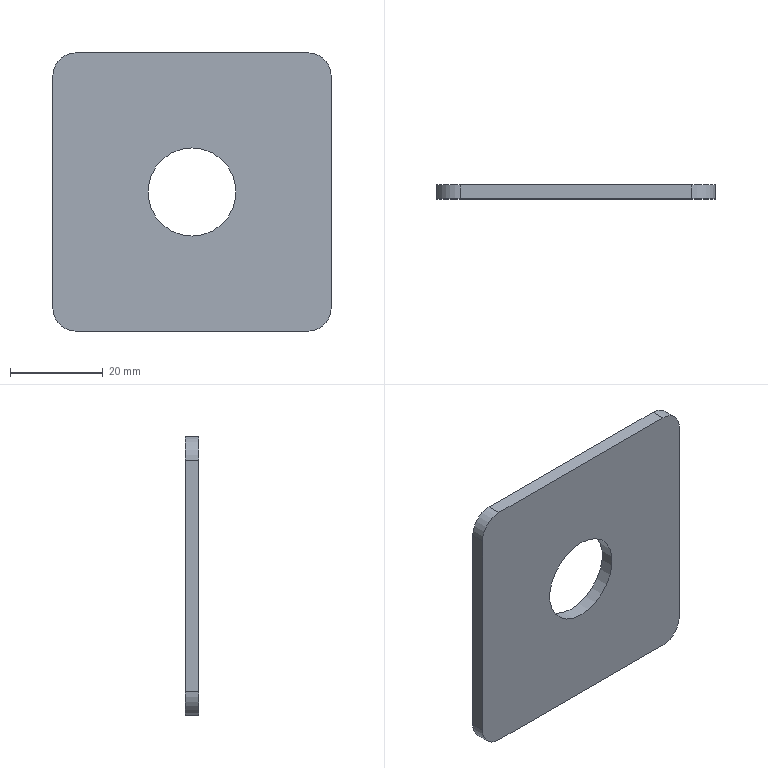Part | STEP file | JBJ-P-1006-04 | 1 solid | 11 faces | box 60 x 3 x 60 mm | volume 9885 mm3 | plane 6 | cylinder 5 | commonest cylinder face diameters 10 x4 19 x1
STEP:
#1=CARTESIAN_POINT('',(60.,3.,55.));
#2=VERTEX_POINT('',#1);
#3=CARTESIAN_POINT('',(60.,3.,5.));
#4=VERTEX_POINT('',#3);
#5=CARTESIAN_POINT('',(60.,3.,0.));
#6=DIRECTION('',(0.,0.,-1.));
#7=VECTOR('',#6,1000.);
#8=LINE('',#5,#7);
#9=EDGE_CURVE('',#2,#4,#8,.T.);
#10=ORIENTED_EDGE('',*,*,#9,.T.);
#11=CARTESIAN_POINT('',(55.,3.,0.));
#12=VERTEX_POINT('',#11);
#13=CARTESIAN_POINT('',(55.,3.,5.));
#14=DIRECTION('',(0.,1.,0.));
#15=DIRECTION('',(0.,0.,1.));
#16=AXIS2_PLACEMENT_3D('',#13,#14,#15);
#17=CIRCLE('',#16,5.);
#18=EDGE_CURVE('',#4,#12,#17,.T.);
#19=ORIENTED_EDGE('',*,*,#18,.T.);
#20=CARTESIAN_POINT('',(5.,3.,0.));
#21=VERTEX_POINT('',#20);
#22=CARTESIAN_POINT('',(0.,3.,0.));
#23=DIRECTION('',(-1.,0.,0.));
#24=VECTOR('',#23,1000.);
#25=LINE('',#22,#24);
#26=EDGE_CURVE('',#12,#21,#25,.T.);
#27=ORIENTED_EDGE('',*,*,#26,.T.);
#28=CARTESIAN_POINT('',(0.,3.,5.));
#29=VERTEX_POINT('',#28);
#30=CARTESIAN_POINT('',(5.,3.,5.));
#31=DIRECTION('',(0.,1.,0.));
#32=DIRECTION('',(0.,0.,1.));
#33=AXIS2_PLACEMENT_3D('',#30,#31,#32);
#34=CIRCLE('',#33,5.);
#35=EDGE_CURVE('',#21,#29,#34,.T.);
#36=ORIENTED_EDGE('',*,*,#35,.T.);
#37=CARTESIAN_POINT('',(0.,3.,55.));
#38=VERTEX_POINT('',#37);
#39=CARTESIAN_POINT('',(0.,3.,0.));
#40=DIRECTION('',(0.,0.,1.));
#41=VECTOR('',#40,1000.);
#42=LINE('',#39,#41);
#43=EDGE_CURVE('',#29,#38,#42,.T.);
#44=ORIENTED_EDGE('',*,*,#43,.T.);
#45=CARTESIAN_POINT('',(5.,3.,60.));
#46=VERTEX_POINT('',#45);
#47=CARTESIAN_POINT('',(5.,3.,55.));
#48=DIRECTION('',(0.,1.,0.));
#49=DIRECTION('',(0.,0.,1.));
#50=AXIS2_PLACEMENT_3D('',#47,#48,#49);
#51=CIRCLE('',#50,5.);
#52=EDGE_CURVE('',#38,#46,#51,.T.);
#53=ORIENTED_EDGE('',*,*,#52,.T.);
#54=CARTESIAN_POINT('',(55.,3.,60.));
#55=VERTEX_POINT('',#54);
#56=CARTESIAN_POINT('',(0.,3.,60.));
#57=DIRECTION('',(1.,0.,0.));
#58=VECTOR('',#57,1000.);
#59=LINE('',#56,#58);
#60=EDGE_CURVE('',#46,#55,#59,.T.);
#61=ORIENTED_EDGE('',*,*,#60,.T.);
#62=CARTESIAN_POINT('',(55.,3.,55.));
#63=DIRECTION('',(0.,1.,0.));
#64=DIRECTION('',(0.,0.,1.));
#65=AXIS2_PLACEMENT_3D('',#62,#63,#64);
#66=CIRCLE('',#65,5.);
#67=EDGE_CURVE('',#55,#2,#66,.T.);
#68=ORIENTED_EDGE('',*,*,#67,.T.);
#69=EDGE_LOOP('',(#10,#19,#27,#36,#44,#53,#61,#68));
#70=FACE_OUTER_BOUND('',#69,.T.);
#71=CARTESIAN_POINT('',(30.,3.,39.5));
#72=VERTEX_POINT('',#71);
#73=CARTESIAN_POINT('',(30.,3.,30.));
#74=DIRECTION('',(0.,1.,0.));
#75=DIRECTION('',(0.,0.,1.));
#76=AXIS2_PLACEMENT_3D('',#73,#74,#75);
#77=CIRCLE('',#76,9.5);
#78=EDGE_CURVE('',#72,#72,#77,.T.);
#79=ORIENTED_EDGE('',*,*,#78,.F.);
#80=EDGE_LOOP('',(#79));
#81=FACE_BOUND('',#80,.T.);
#82=CARTESIAN_POINT('',(0.,3.,0.));
#83=DIRECTION('',(0.,1.,0.));
#84=DIRECTION('',(0.,0.,1.));
#85=AXIS2_PLACEMENT_3D('',#82,#83,#84);
#86=PLANE('',#85);
#87=ADVANCED_FACE('',(#70,#81),#86,.T.);
#88=CARTESIAN_POINT('',(55.,0.,0.));
#89=VERTEX_POINT('',#88);
#90=CARTESIAN_POINT('',(5.,0.,0.));
#91=VERTEX_POINT('',#90);
#92=CARTESIAN_POINT('',(0.,0.,0.));
#93=DIRECTION('',(-1.,0.,0.));
#94=VECTOR('',#93,1000.);
#95=LINE('',#92,#94);
#96=EDGE_CURVE('',#89,#91,#95,.T.);
#97=ORIENTED_EDGE('',*,*,#96,.F.);
#98=CARTESIAN_POINT('',(60.,0.,5.));
#99=VERTEX_POINT('',#98);
#100=CARTESIAN_POINT('',(55.,0.,5.));
#101=DIRECTION('',(0.,-1.,0.));
#102=DIRECTION('',(0.,0.,1.));
#103=AXIS2_PLACEMENT_3D('',#100,#101,#102);
#104=CIRCLE('',#103,5.);
#105=EDGE_CURVE('',#89,#99,#104,.T.);
#106=ORIENTED_EDGE('',*,*,#105,.T.);
#107=CARTESIAN_POINT('',(60.,0.,55.));
#108=VERTEX_POINT('',#107);
#109=CARTESIAN_POINT('',(60.,0.,0.));
#110=DIRECTION('',(0.,0.,-1.));
#111=VECTOR('',#110,1000.);
#112=LINE('',#109,#111);
#113=EDGE_CURVE('',#108,#99,#112,.T.);
#114=ORIENTED_EDGE('',*,*,#113,.F.);
#115=CARTESIAN_POINT('',(55.,0.,60.));
#116=VERTEX_POINT('',#115);
#117=CARTESIAN_POINT('',(55.,0.,55.));
#118=DIRECTION('',(0.,-1.,0.));
#119=DIRECTION('',(0.,0.,1.));
#120=AXIS2_PLACEMENT_3D('',#117,#118,#119);
#121=CIRCLE('',#120,5.);
#122=EDGE_CURVE('',#108,#116,#121,.T.);
#123=ORIENTED_EDGE('',*,*,#122,.T.);
#124=CARTESIAN_POINT('',(5.,0.,60.));
#125=VERTEX_POINT('',#124);
#126=CARTESIAN_POINT('',(0.,0.,60.));
#127=DIRECTION('',(1.,0.,0.));
#128=VECTOR('',#127,1000.);
#129=LINE('',#126,#128);
#130=EDGE_CURVE('',#125,#116,#129,.T.);
#131=ORIENTED_EDGE('',*,*,#130,.F.);
#132=CARTESIAN_POINT('',(0.,0.,55.));
#133=VERTEX_POINT('',#132);
#134=CARTESIAN_POINT('',(5.,0.,55.));
#135=DIRECTION('',(0.,-1.,0.));
#136=DIRECTION('',(0.,0.,1.));
#137=AXIS2_PLACEMENT_3D('',#134,#135,#136);
#138=CIRCLE('',#137,5.);
#139=EDGE_CURVE('',#125,#133,#138,.T.);
#140=ORIENTED_EDGE('',*,*,#139,.T.);
#141=CARTESIAN_POINT('',(0.,0.,5.));
#142=VERTEX_POINT('',#141);
#143=CARTESIAN_POINT('',(0.,0.,0.));
#144=DIRECTION('',(0.,0.,1.));
#145=VECTOR('',#144,1000.);
#146=LINE('',#143,#145);
#147=EDGE_CURVE('',#142,#133,#146,.T.);
#148=ORIENTED_EDGE('',*,*,#147,.F.);
#149=CARTESIAN_POINT('',(5.,0.,5.));
#150=DIRECTION('',(0.,-1.,0.));
#151=DIRECTION('',(0.,0.,1.));
#152=AXIS2_PLACEMENT_3D('',#149,#150,#151);
#153=CIRCLE('',#152,5.);
#154=EDGE_CURVE('',#142,#91,#153,.T.);
#155=ORIENTED_EDGE('',*,*,#154,.T.);
#156=EDGE_LOOP('',(#97,#106,#114,#123,#131,#140,#148,#155));
#157=FACE_OUTER_BOUND('',#156,.T.);
#158=CARTESIAN_POINT('',(30.,0.,39.5));
#159=VERTEX_POINT('',#158);
#160=CARTESIAN_POINT('',(30.,0.,30.));
#161=DIRECTION('',(0.,1.,0.));
#162=DIRECTION('',(0.,0.,1.));
#163=AXIS2_PLACEMENT_3D('',#160,#161,#162);
#164=CIRCLE('',#163,9.5);
#165=EDGE_CURVE('',#159,#159,#164,.T.);
#166=ORIENTED_EDGE('',*,*,#165,.T.);
#167=EDGE_LOOP('',(#166));
#168=FACE_BOUND('',#167,.T.);
#169=CARTESIAN_POINT('',(0.,0.,0.));
#170=DIRECTION('',(0.,1.,0.));
#171=DIRECTION('',(0.,0.,1.));
#172=AXIS2_PLACEMENT_3D('',#169,#170,#171);
#173=PLANE('',#172);
#174=ADVANCED_FACE('',(#157,#168),#173,.F.);
#175=ORIENTED_EDGE('',*,*,#43,.F.);
#176=CARTESIAN_POINT('',(0.,3.,5.));
#177=DIRECTION('',(0.,-1.,0.));
#178=VECTOR('',#177,1000.);
#179=LINE('',#176,#178);
#180=EDGE_CURVE('',#29,#142,#179,.T.);
#181=ORIENTED_EDGE('',*,*,#180,.T.);
#182=ORIENTED_EDGE('',*,*,#147,.T.);
#183=CARTESIAN_POINT('',(0.,3.,55.));
#184=DIRECTION('',(0.,1.,0.));
#185=VECTOR('',#184,1000.);
#186=LINE('',#183,#185);
#187=EDGE_CURVE('',#133,#38,#186,.T.);
#188=ORIENTED_EDGE('',*,*,#187,.T.);
#189=EDGE_LOOP('',(#175,#181,#182,#188));
#190=FACE_OUTER_BOUND('',#189,.T.);
#191=CARTESIAN_POINT('',(0.,3.,0.));
#192=DIRECTION('',(1.,0.,0.));
#193=DIRECTION('',(0.,0.,-1.));
#194=AXIS2_PLACEMENT_3D('',#191,#192,#193);
#195=PLANE('',#194);
#196=ADVANCED_FACE('',(#190),#195,.F.);
#197=ORIENTED_EDGE('',*,*,#60,.F.);
#198=CARTESIAN_POINT('',(5.,3.,60.));
#199=DIRECTION('',(0.,-1.,0.));
#200=VECTOR('',#199,1000.);
#201=LINE('',#198,#200);
#202=EDGE_CURVE('',#46,#125,#201,.T.);
#203=ORIENTED_EDGE('',*,*,#202,.T.);
#204=ORIENTED_EDGE('',*,*,#130,.T.);
#205=CARTESIAN_POINT('',(55.,3.,60.));
#206=DIRECTION('',(0.,1.,0.));
#207=VECTOR('',#206,1000.);
#208=LINE('',#205,#207);
#209=EDGE_CURVE('',#116,#55,#208,.T.);
#210=ORIENTED_EDGE('',*,*,#209,.T.);
#211=EDGE_LOOP('',(#197,#203,#204,#210));
#212=FACE_OUTER_BOUND('',#211,.T.);
#213=CARTESIAN_POINT('',(0.,3.,60.));
#214=DIRECTION('',(0.,0.,-1.));
#215=DIRECTION('',(-1.,0.,0.));
#216=AXIS2_PLACEMENT_3D('',#213,#214,#215);
#217=PLANE('',#216);
#218=ADVANCED_FACE('',(#212),#217,.F.);
#219=ORIENTED_EDGE('',*,*,#113,.T.);
#220=CARTESIAN_POINT('',(60.,3.,5.));
#221=DIRECTION('',(0.,1.,0.));
#222=VECTOR('',#221,1000.);
#223=LINE('',#220,#222);
#224=EDGE_CURVE('',#99,#4,#223,.T.);
#225=ORIENTED_EDGE('',*,*,#224,.T.);
#226=ORIENTED_EDGE('',*,*,#9,.F.);
#227=CARTESIAN_POINT('',(60.,3.,55.));
#228=DIRECTION('',(0.,-1.,0.));
#229=VECTOR('',#228,1000.);
#230=LINE('',#227,#229);
#231=EDGE_CURVE('',#2,#108,#230,.T.);
#232=ORIENTED_EDGE('',*,*,#231,.T.);
#233=EDGE_LOOP('',(#219,#225,#226,#232));
#234=FACE_OUTER_BOUND('',#233,.T.);
#235=CARTESIAN_POINT('',(60.,3.,0.));
#236=DIRECTION('',(-1.,0.,0.));
#237=DIRECTION('',(0.,0.,1.));
#238=AXIS2_PLACEMENT_3D('',#235,#236,#237);
#239=PLANE('',#238);
#240=ADVANCED_FACE('',(#234),#239,.F.);
#241=ORIENTED_EDGE('',*,*,#26,.F.);
#242=CARTESIAN_POINT('',(55.,3.,0.));
#243=DIRECTION('',(0.,-1.,0.));
#244=VECTOR('',#243,1000.);
#245=LINE('',#242,#244);
#246=EDGE_CURVE('',#12,#89,#245,.T.);
#247=ORIENTED_EDGE('',*,*,#246,.T.);
#248=ORIENTED_EDGE('',*,*,#96,.T.);
#249=CARTESIAN_POINT('',(5.,3.,0.));
#250=DIRECTION('',(0.,1.,0.));
#251=VECTOR('',#250,1000.);
#252=LINE('',#249,#251);
#253=EDGE_CURVE('',#91,#21,#252,.T.);
#254=ORIENTED_EDGE('',*,*,#253,.T.);
#255=EDGE_LOOP('',(#241,#247,#248,#254));
#256=FACE_OUTER_BOUND('',#255,.T.);
#257=CARTESIAN_POINT('',(0.,3.,0.));
#258=DIRECTION('',(0.,0.,1.));
#259=DIRECTION('',(1.,0.,0.));
#260=AXIS2_PLACEMENT_3D('',#257,#258,#259);
#261=PLANE('',#260);
#262=ADVANCED_FACE('',(#256),#261,.F.);
#263=ORIENTED_EDGE('',*,*,#78,.T.);
#264=EDGE_LOOP('',(#263));
#265=FACE_OUTER_BOUND('',#264,.T.);
#266=ORIENTED_EDGE('',*,*,#165,.F.);
#267=EDGE_LOOP('',(#266));
#268=FACE_OUTER_BOUND('',#267,.T.);
#269=CARTESIAN_POINT('',(30.,3.,30.));
#270=DIRECTION('',(0.,-1.,0.));
#271=DIRECTION('',(0.,0.,-1.));
#272=AXIS2_PLACEMENT_3D('',#269,#270,#271);
#273=CYLINDRICAL_SURFACE('',#272,9.5);
#274=ADVANCED_FACE('',(#265,#268),#273,.F.);
#275=ORIENTED_EDGE('',*,*,#18,.F.);
#276=ORIENTED_EDGE('',*,*,#224,.F.);
#277=ORIENTED_EDGE('',*,*,#105,.F.);
#278=ORIENTED_EDGE('',*,*,#246,.F.);
#279=EDGE_LOOP('',(#275,#276,#277,#278));
#280=FACE_OUTER_BOUND('',#279,.T.);
#281=CARTESIAN_POINT('',(55.,3.,5.));
#282=DIRECTION('',(0.,-1.,0.));
#283=DIRECTION('',(0.,0.,-1.));
#284=AXIS2_PLACEMENT_3D('',#281,#282,#283);
#285=CYLINDRICAL_SURFACE('',#284,5.);
#286=ADVANCED_FACE('',(#280),#285,.T.);
#287=ORIENTED_EDGE('',*,*,#35,.F.);
#288=ORIENTED_EDGE('',*,*,#253,.F.);
#289=ORIENTED_EDGE('',*,*,#154,.F.);
#290=ORIENTED_EDGE('',*,*,#180,.F.);
#291=EDGE_LOOP('',(#287,#288,#289,#290));
#292=FACE_OUTER_BOUND('',#291,.T.);
#293=CARTESIAN_POINT('',(5.,3.,5.));
#294=DIRECTION('',(0.,-1.,0.));
#295=DIRECTION('',(0.,0.,-1.));
#296=AXIS2_PLACEMENT_3D('',#293,#294,#295);
#297=CYLINDRICAL_SURFACE('',#296,5.);
#298=ADVANCED_FACE('',(#292),#297,.T.);
#299=ORIENTED_EDGE('',*,*,#52,.F.);
#300=ORIENTED_EDGE('',*,*,#187,.F.);
#301=ORIENTED_EDGE('',*,*,#139,.F.);
#302=ORIENTED_EDGE('',*,*,#202,.F.);
#303=EDGE_LOOP('',(#299,#300,#301,#302));
#304=FACE_OUTER_BOUND('',#303,.T.);
#305=CARTESIAN_POINT('',(5.,3.,55.));
#306=DIRECTION('',(0.,-1.,0.));
#307=DIRECTION('',(0.,0.,-1.));
#308=AXIS2_PLACEMENT_3D('',#305,#306,#307);
#309=CYLINDRICAL_SURFACE('',#308,5.);
#310=ADVANCED_FACE('',(#304),#309,.T.);
#311=ORIENTED_EDGE('',*,*,#67,.F.);
#312=ORIENTED_EDGE('',*,*,#209,.F.);
#313=ORIENTED_EDGE('',*,*,#122,.F.);
#314=ORIENTED_EDGE('',*,*,#231,.F.);
#315=EDGE_LOOP('',(#311,#312,#313,#314));
#316=FACE_OUTER_BOUND('',#315,.T.);
#317=CARTESIAN_POINT('',(55.,3.,55.));
#318=DIRECTION('',(0.,-1.,0.));
#319=DIRECTION('',(0.,0.,-1.));
#320=AXIS2_PLACEMENT_3D('',#317,#318,#319);
#321=CYLINDRICAL_SURFACE('',#320,5.);
#322=ADVANCED_FACE('',(#316),#321,.T.);
#323=CLOSED_SHELL('',(#87,#174,#196,#218,#240,#262,#274,#286,#298,#310,#322));
#324=MANIFOLD_SOLID_BREP('',#323);
#325=CARTESIAN_POINT('',(0.,0.,0.));
#326=DIRECTION('',(0.,0.,1.));
#327=DIRECTION('',(1.,0.,0.));
#328=AXIS2_PLACEMENT_3D('',#325,#326,#327);
#329=(LENGTH_UNIT()NAMED_UNIT(*)SI_UNIT(.MILLI.,.METRE.));
#330=UNCERTAINTY_MEASURE_WITH_UNIT(LENGTH_MEASURE(0.00001),#329,'','');
#331=(NAMED_UNIT(*)PLANE_ANGLE_UNIT()SI_UNIT($,.RADIAN.));
#332=(NAMED_UNIT(*)SI_UNIT($,.STERADIAN.)SOLID_ANGLE_UNIT());
#333=(GEOMETRIC_REPRESENTATION_CONTEXT(3)GLOBAL_UNCERTAINTY_ASSIGNED_CONTEXT((#330))GLOBAL_UNIT_ASSIGNED_CONTEXT((#329,#331,#332))REPRESENTATION_CONTEXT('',''));
#334=ADVANCED_BREP_SHAPE_REPRESENTATION('',(#324,#328),#333);